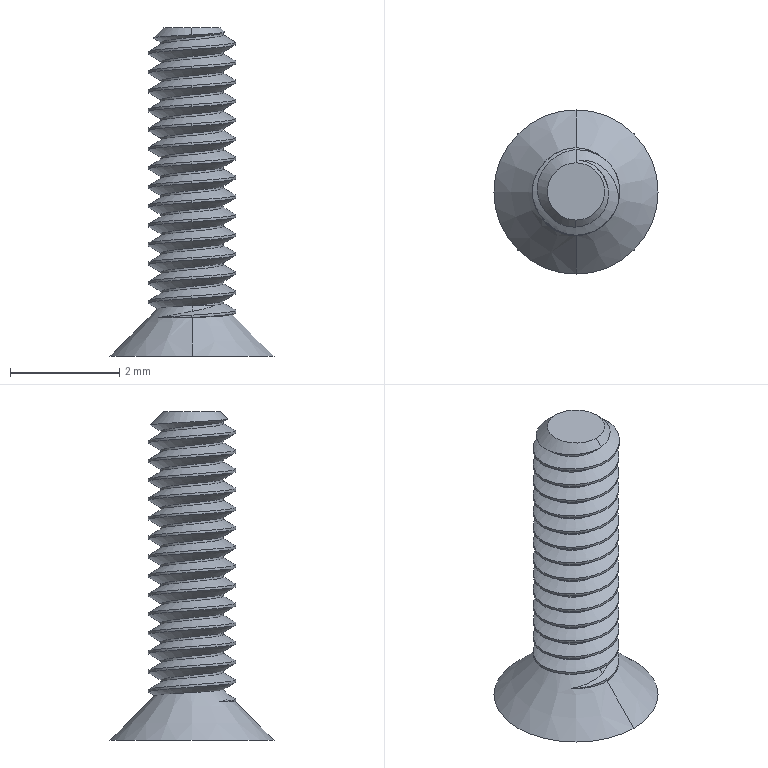Part | NX | features solid 2 | 1 solid | 64 faces | box 3 x 3 x 6 mm | volume 10.563 mm3 | cylinder 37 | plane 19 | cone 5 | spline 3 | commonest cylinder face diameters 1.6 x30 1.854 x7